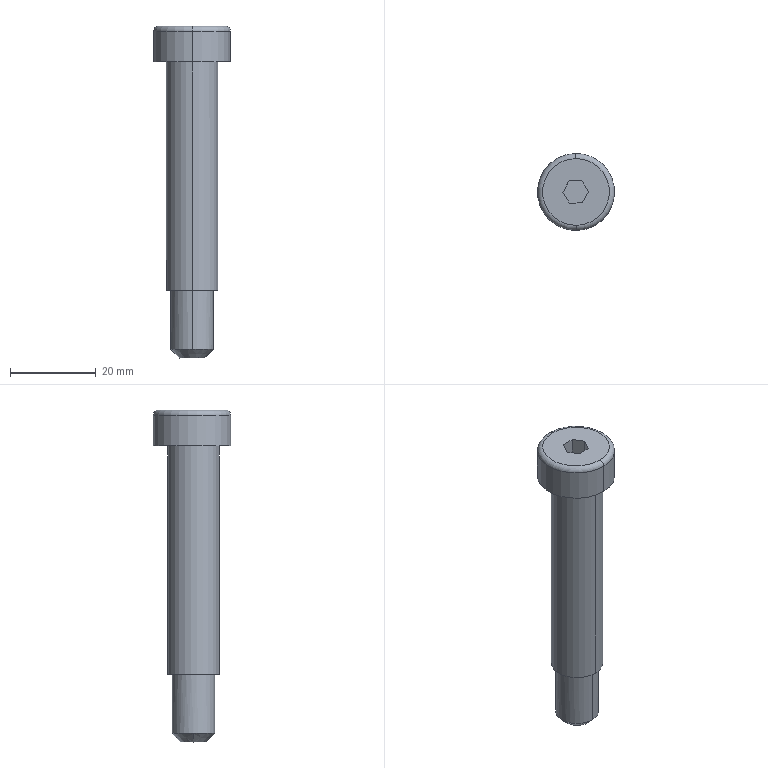Part | SolidWorks | features BaseBody 1 | 1 solid | 21 faces | box 18.001 x 18 x 77.489 mm | volume 9192 mm3 | plane 11 | cylinder 6 | torus 2 | cone 2 | commonest cylinder face diameters 10 x2 12 x2 18 x2
STEP:
#1=CARTESIAN_POINT('',(341.564,206.739,62.122));
#2=VERTEX_POINT('',#1);
#3=CARTESIAN_POINT('',(341.942,188.743,62.122));
#4=VERTEX_POINT('',#3);
#5=CARTESIAN_POINT('',(341.753,197.741,62.122));
#6=DIRECTION('',(-0.0001435,-0.000000521,1.));
#7=DIRECTION('',(0.02104,-0.9998,0.000002497));
#8=AXIS2_PLACEMENT_3D('',#5,#6,#7);
#9=CIRCLE('',#8,9.);
#10=EDGE_CURVE('',#2,#4,#9,.T.);
#11=ORIENTED_EDGE('',*,*,#10,.T.);
#12=CARTESIAN_POINT('',(341.917,189.943,63.322));
#13=VERTEX_POINT('',#12);
#14=CARTESIAN_POINT('',(341.917,189.943,62.122));
#15=DIRECTION('',(-0.9998,-0.02104,-0.0001435));
#16=DIRECTION('',(0.02104,-0.9998,0.));
#17=AXIS2_PLACEMENT_3D('',#14,#15,#16);
#18=CIRCLE('',#17,1.2);
#19=EDGE_CURVE('',#4,#13,#18,.T.);
#20=ORIENTED_EDGE('',*,*,#19,.T.);
#21=CARTESIAN_POINT('',(341.589,205.539,63.322));
#22=VERTEX_POINT('',#21);
#23=CARTESIAN_POINT('',(341.753,197.741,63.322));
#24=DIRECTION('',(-0.0001435,-0.000000521,1.));
#25=DIRECTION('',(0.02104,-0.9998,0.000002497));
#26=AXIS2_PLACEMENT_3D('',#23,#24,#25);
#27=CIRCLE('',#26,7.8);
#28=EDGE_CURVE('',#22,#13,#27,.T.);
#29=ORIENTED_EDGE('',*,*,#28,.F.);
#30=CARTESIAN_POINT('',(341.589,205.539,62.122));
#31=DIRECTION('',(0.9998,0.02104,0.0001435));
#32=DIRECTION('',(-0.02104,0.9998,0.));
#33=AXIS2_PLACEMENT_3D('',#30,#31,#32);
#34=CIRCLE('',#33,1.2);
#35=EDGE_CURVE('',#2,#22,#34,.T.);
#36=ORIENTED_EDGE('',*,*,#35,.F.);
#37=EDGE_LOOP('',(#11,#20,#29,#36));
#38=FACE_OUTER_BOUND('',#37,.T.);
#39=CARTESIAN_POINT('',(341.753,197.741,62.122));
#40=DIRECTION('',(-0.0001435,-0.000000521,1.));
#41=DIRECTION('',(-0.02104,0.9998,-0.000002497));
#42=AXIS2_PLACEMENT_3D('',#39,#40,#41);
#43=TOROIDAL_SURFACE('',#42,7.8,1.2);
#44=ADVANCED_FACE('',(#38),#43,.T.);
#45=CARTESIAN_POINT('',(341.943,188.743,54.922));
#46=VERTEX_POINT('',#45);
#47=CARTESIAN_POINT('',(341.565,206.739,54.922));
#48=VERTEX_POINT('',#47);
#49=CARTESIAN_POINT('',(341.754,197.741,54.922));
#50=DIRECTION('',(0.0001435,0.000000521,-1.));
#51=DIRECTION('',(-0.02104,0.9998,-0.000002497));
#52=AXIS2_PLACEMENT_3D('',#49,#50,#51);
#53=CIRCLE('',#52,9.);
#54=EDGE_CURVE('',#46,#48,#53,.T.);
#55=ORIENTED_EDGE('',*,*,#54,.F.);
#56=CARTESIAN_POINT('',(341.943,188.743,54.922));
#57=DIRECTION('',(-0.0001435,-0.000000521,1.));
#58=VECTOR('',#57,1000.);
#59=LINE('',#56,#58);
#60=EDGE_CURVE('',#46,#4,#59,.T.);
#61=ORIENTED_EDGE('',*,*,#60,.T.);
#62=ORIENTED_EDGE('',*,*,#10,.F.);
#63=CARTESIAN_POINT('',(341.565,206.739,54.922));
#64=DIRECTION('',(-0.0001435,-0.000000521,1.));
#65=VECTOR('',#64,1000.);
#66=LINE('',#63,#65);
#67=EDGE_CURVE('',#48,#2,#66,.T.);
#68=ORIENTED_EDGE('',*,*,#67,.F.);
#69=EDGE_LOOP('',(#55,#61,#62,#68));
#70=FACE_OUTER_BOUND('',#69,.T.);
#71=CARTESIAN_POINT('',(341.754,197.741,54.922));
#72=DIRECTION('',(-0.0001435,-0.000000521,1.));
#73=DIRECTION('',(-0.02104,0.9998,-0.000002497));
#74=AXIS2_PLACEMENT_3D('',#71,#72,#73);
#75=CYLINDRICAL_SURFACE('',#74,9.);
#76=ADVANCED_FACE('',(#70),#75,.T.);
#77=CARTESIAN_POINT('',(341.638,203.402,54.922));
#78=VERTEX_POINT('',#77);
#79=CARTESIAN_POINT('',(341.89,191.405,54.922));
#80=VERTEX_POINT('',#79);
#81=CARTESIAN_POINT('',(341.764,197.404,54.922));
#82=DIRECTION('',(-0.0001435,-0.000000521,1.));
#83=DIRECTION('',(0.02104,-0.9998,0.000002497));
#84=AXIS2_PLACEMENT_3D('',#81,#82,#83);
#85=CIRCLE('',#84,6.);
#86=EDGE_CURVE('',#78,#80,#85,.T.);
#87=ORIENTED_EDGE('',*,*,#86,.F.);
#88=CARTESIAN_POINT('',(341.645,203.402,1.675));
#89=VERTEX_POINT('',#88);
#90=CARTESIAN_POINT('',(341.643,203.402,20.275));
#91=DIRECTION('',(0.0001435,0.000000521,-1.));
#92=VECTOR('',#91,1000.);
#93=LINE('',#90,#92);
#94=EDGE_CURVE('',#78,#89,#93,.T.);
#95=ORIENTED_EDGE('',*,*,#94,.T.);
#96=CARTESIAN_POINT('',(341.898,191.405,1.675));
#97=VERTEX_POINT('',#96);
#98=CARTESIAN_POINT('',(341.771,197.404,1.675));
#99=DIRECTION('',(0.0001435,0.000000521,-1.));
#100=DIRECTION('',(0.02104,-0.9998,0.000002497));
#101=AXIS2_PLACEMENT_3D('',#98,#99,#100);
#102=CIRCLE('',#101,6.);
#103=EDGE_CURVE('',#97,#89,#102,.T.);
#104=ORIENTED_EDGE('',*,*,#103,.F.);
#105=CARTESIAN_POINT('',(341.895,191.405,20.275));
#106=DIRECTION('',(0.0001435,0.000000521,-1.));
#107=VECTOR('',#106,1000.);
#108=LINE('',#105,#107);
#109=EDGE_CURVE('',#80,#97,#108,.T.);
#110=ORIENTED_EDGE('',*,*,#109,.F.);
#111=EDGE_LOOP('',(#87,#95,#104,#110));
#112=FACE_OUTER_BOUND('',#111,.T.);
#113=CARTESIAN_POINT('',(341.769,197.404,20.275));
#114=DIRECTION('',(0.0001435,0.000000521,-1.));
#115=DIRECTION('',(0.02104,-0.9998,0.000002497));
#116=AXIS2_PLACEMENT_3D('',#113,#114,#115);
#117=CYLINDRICAL_SURFACE('',#116,6.);
#118=ADVANCED_FACE('',(#112),#117,.T.);
#119=CARTESIAN_POINT('',(341.666,202.402,1.675));
#120=VERTEX_POINT('',#119);
#121=CARTESIAN_POINT('',(341.877,192.405,1.675));
#122=VERTEX_POINT('',#121);
#123=CARTESIAN_POINT('',(341.771,197.404,1.675));
#124=DIRECTION('',(-0.0001435,-0.000000521,1.));
#125=DIRECTION('',(0.02104,-0.9998,0.000002497));
#126=AXIS2_PLACEMENT_3D('',#123,#124,#125);
#127=CIRCLE('',#126,5.);
#128=EDGE_CURVE('',#120,#122,#127,.T.);
#129=ORIENTED_EDGE('',*,*,#128,.F.);
#130=CARTESIAN_POINT('',(341.668,202.402,-12.165));
#131=VERTEX_POINT('',#130);
#132=CARTESIAN_POINT('',(341.667,202.402,-0.7255));
#133=DIRECTION('',(0.0001435,0.000000521,-1.));
#134=VECTOR('',#133,1000.);
#135=LINE('',#132,#134);
#136=EDGE_CURVE('',#120,#131,#135,.T.);
#137=ORIENTED_EDGE('',*,*,#136,.T.);
#138=CARTESIAN_POINT('',(336.773,197.404,-12.166));
#139=VERTEX_POINT('',#138);
#140=CARTESIAN_POINT('',(341.773,197.404,-12.165));
#141=DIRECTION('',(0.0001435,0.000000521,-1.));
#142=DIRECTION('',(0.02104,-0.9998,0.000002497));
#143=AXIS2_PLACEMENT_3D('',#140,#141,#142);
#144=CIRCLE('',#143,5.);
#145=EDGE_CURVE('',#139,#131,#144,.T.);
#146=ORIENTED_EDGE('',*,*,#145,.F.);
#147=CARTESIAN_POINT('',(341.879,192.405,-12.165));
#148=VERTEX_POINT('',#147);
#149=CARTESIAN_POINT('',(341.773,197.404,-12.165));
#150=DIRECTION('',(0.0001435,0.000000521,-1.));
#151=DIRECTION('',(0.02104,-0.9998,0.000002497));
#152=AXIS2_PLACEMENT_3D('',#149,#150,#151);
#153=CIRCLE('',#152,5.);
#154=EDGE_CURVE('',#148,#139,#153,.T.);
#155=ORIENTED_EDGE('',*,*,#154,.F.);
#156=CARTESIAN_POINT('',(341.877,192.405,-0.7254));
#157=DIRECTION('',(0.0001435,0.000000521,-1.));
#158=VECTOR('',#157,1000.);
#159=LINE('',#156,#158);
#160=EDGE_CURVE('',#122,#148,#159,.T.);
#161=ORIENTED_EDGE('',*,*,#160,.F.);
#162=EDGE_LOOP('',(#129,#137,#146,#155,#161));
#163=FACE_OUTER_BOUND('',#162,.T.);
#164=CARTESIAN_POINT('',(341.772,197.404,-0.7254));
#165=DIRECTION('',(0.0001435,0.000000521,-1.));
#166=DIRECTION('',(0.02104,-0.9998,0.000002497));
#167=AXIS2_PLACEMENT_3D('',#164,#165,#166);
#168=CYLINDRICAL_SURFACE('',#167,5.);
#169=ADVANCED_FACE('',(#163),#168,.T.);
#170=CARTESIAN_POINT('',(338.774,197.404,-14.166));
#171=VERTEX_POINT('',#170);
#172=CARTESIAN_POINT('',(344.774,197.404,-14.165));
#173=VERTEX_POINT('',#172);
#174=CARTESIAN_POINT('',(341.774,197.404,-14.165));
#175=DIRECTION('',(0.0001435,0.000000521,-1.));
#176=DIRECTION('',(-1.,0.,-0.0001435));
#177=AXIS2_PLACEMENT_3D('',#174,#175,#176);
#178=CIRCLE('',#177,3.);
#179=EDGE_CURVE('',#171,#173,#178,.T.);
#180=ORIENTED_EDGE('',*,*,#179,.F.);
#181=CARTESIAN_POINT('',(337.774,197.404,-13.166));
#182=DIRECTION('',(-0.7072,-0.000000369,0.707));
#183=VECTOR('',#182,1000.);
#184=LINE('',#181,#183);
#185=EDGE_CURVE('',#171,#139,#184,.T.);
#186=ORIENTED_EDGE('',*,*,#185,.T.);
#187=ORIENTED_EDGE('',*,*,#145,.T.);
#188=CARTESIAN_POINT('',(346.773,197.404,-12.165));
#189=VERTEX_POINT('',#188);
#190=CARTESIAN_POINT('',(341.773,197.404,-12.165));
#191=DIRECTION('',(0.0001435,0.000000521,-1.));
#192=DIRECTION('',(0.02104,-0.9998,0.000002497));
#193=AXIS2_PLACEMENT_3D('',#190,#191,#192);
#194=CIRCLE('',#193,5.);
#195=EDGE_CURVE('',#131,#189,#194,.T.);
#196=ORIENTED_EDGE('',*,*,#195,.T.);
#197=CARTESIAN_POINT('',(345.774,197.404,-13.165));
#198=DIRECTION('',(0.707,-0.000000369,0.7072));
#199=VECTOR('',#198,1000.);
#200=LINE('',#197,#199);
#201=EDGE_CURVE('',#173,#189,#200,.T.);
#202=ORIENTED_EDGE('',*,*,#201,.F.);
#203=EDGE_LOOP('',(#180,#186,#187,#196,#202));
#204=FACE_OUTER_BOUND('',#203,.T.);
#205=CARTESIAN_POINT('',(341.774,197.404,-13.165));
#206=DIRECTION('',(-0.0001435,-0.000000521,1.));
#207=DIRECTION('',(1.,0.,0.0001435));
#208=AXIS2_PLACEMENT_3D('',#205,#206,#207);
#209=CONICAL_SURFACE('',#208,4.,0.7854);
#210=ADVANCED_FACE('',(#204),#209,.T.);
#211=CARTESIAN_POINT('',(341.774,197.404,-14.165));
#212=DIRECTION('',(0.0001435,0.000000521,-1.));
#213=DIRECTION('',(-1.,0.,-0.0001435));
#214=AXIS2_PLACEMENT_3D('',#211,#212,#213);
#215=CIRCLE('',#214,3.);
#216=EDGE_CURVE('',#173,#171,#215,.T.);
#217=ORIENTED_EDGE('',*,*,#216,.T.);
#218=ORIENTED_EDGE('',*,*,#179,.T.);
#219=EDGE_LOOP('',(#217,#218));
#220=FACE_OUTER_BOUND('',#219,.T.);
#221=CARTESIAN_POINT('',(341.774,197.404,-14.165));
#222=DIRECTION('',(0.0001435,0.000000521,-1.));
#223=DIRECTION('',(0.,-1.,-0.000000521));
#224=AXIS2_PLACEMENT_3D('',#221,#222,#223);
#225=PLANE('',#224);
#226=ADVANCED_FACE('',(#220),#225,.T.);
#227=ORIENTED_EDGE('',*,*,#185,.F.);
#228=ORIENTED_EDGE('',*,*,#216,.F.);
#229=ORIENTED_EDGE('',*,*,#201,.T.);
#230=CARTESIAN_POINT('',(341.773,197.404,-12.165));
#231=DIRECTION('',(0.0001435,0.000000521,-1.));
#232=DIRECTION('',(0.02104,-0.9998,0.000002497));
#233=AXIS2_PLACEMENT_3D('',#230,#231,#232);
#234=CIRCLE('',#233,5.);
#235=EDGE_CURVE('',#189,#148,#234,.T.);
#236=ORIENTED_EDGE('',*,*,#235,.T.);
#237=ORIENTED_EDGE('',*,*,#154,.T.);
#238=EDGE_LOOP('',(#227,#228,#229,#236,#237));
#239=FACE_OUTER_BOUND('',#238,.T.);
#240=CARTESIAN_POINT('',(341.774,197.404,-13.165));
#241=DIRECTION('',(-0.0001435,-0.000000521,1.));
#242=DIRECTION('',(1.,0.,0.0001435));
#243=AXIS2_PLACEMENT_3D('',#240,#241,#242);
#244=CONICAL_SURFACE('',#243,4.,0.7854);
#245=ADVANCED_FACE('',(#239),#244,.T.);
#246=ORIENTED_EDGE('',*,*,#136,.F.);
#247=CARTESIAN_POINT('',(341.771,197.404,1.675));
#248=DIRECTION('',(-0.0001435,-0.000000521,1.));
#249=DIRECTION('',(0.02104,-0.9998,0.000002497));
#250=AXIS2_PLACEMENT_3D('',#247,#248,#249);
#251=CIRCLE('',#250,5.);
#252=EDGE_CURVE('',#122,#120,#251,.T.);
#253=ORIENTED_EDGE('',*,*,#252,.F.);
#254=ORIENTED_EDGE('',*,*,#160,.T.);
#255=ORIENTED_EDGE('',*,*,#235,.F.);
#256=ORIENTED_EDGE('',*,*,#195,.F.);
#257=EDGE_LOOP('',(#246,#253,#254,#255,#256));
#258=FACE_OUTER_BOUND('',#257,.T.);
#259=CARTESIAN_POINT('',(341.772,197.404,-0.7254));
#260=DIRECTION('',(0.0001435,0.000000521,-1.));
#261=DIRECTION('',(0.02104,-0.9998,0.000002497));
#262=AXIS2_PLACEMENT_3D('',#259,#260,#261);
#263=CYLINDRICAL_SURFACE('',#262,5.);
#264=ADVANCED_FACE('',(#258),#263,.T.);
#265=ORIENTED_EDGE('',*,*,#252,.T.);
#266=ORIENTED_EDGE('',*,*,#128,.T.);
#267=EDGE_LOOP('',(#265,#266));
#268=FACE_BOUND('',#267,.T.);
#269=ORIENTED_EDGE('',*,*,#103,.T.);
#270=CARTESIAN_POINT('',(341.771,197.404,1.675));
#271=DIRECTION('',(0.0001435,0.000000521,-1.));
#272=DIRECTION('',(0.02104,-0.9998,0.000002497));
#273=AXIS2_PLACEMENT_3D('',#270,#271,#272);
#274=CIRCLE('',#273,6.);
#275=EDGE_CURVE('',#89,#97,#274,.T.);
#276=ORIENTED_EDGE('',*,*,#275,.T.);
#277=EDGE_LOOP('',(#269,#276));
#278=FACE_OUTER_BOUND('',#277,.T.);
#279=CARTESIAN_POINT('',(341.771,197.404,1.675));
#280=DIRECTION('',(0.0001435,0.000000521,-1.));
#281=DIRECTION('',(0.,-1.,-0.000000521));
#282=AXIS2_PLACEMENT_3D('',#279,#280,#281);
#283=PLANE('',#282);
#284=ADVANCED_FACE('',(#268,#278),#283,.T.);
#285=ORIENTED_EDGE('',*,*,#94,.F.);
#286=CARTESIAN_POINT('',(341.764,197.404,54.922));
#287=DIRECTION('',(-0.0001435,-0.000000521,1.));
#288=DIRECTION('',(0.02104,-0.9998,0.000002497));
#289=AXIS2_PLACEMENT_3D('',#286,#287,#288);
#290=CIRCLE('',#289,6.);
#291=EDGE_CURVE('',#80,#78,#290,.T.);
#292=ORIENTED_EDGE('',*,*,#291,.F.);
#293=ORIENTED_EDGE('',*,*,#109,.T.);
#294=ORIENTED_EDGE('',*,*,#275,.F.);
#295=EDGE_LOOP('',(#285,#292,#293,#294));
#296=FACE_OUTER_BOUND('',#295,.T.);
#297=CARTESIAN_POINT('',(341.769,197.404,20.275));
#298=DIRECTION('',(0.0001435,0.000000521,-1.));
#299=DIRECTION('',(0.02104,-0.9998,0.000002497));
#300=AXIS2_PLACEMENT_3D('',#297,#298,#299);
#301=CYLINDRICAL_SURFACE('',#300,6.);
#302=ADVANCED_FACE('',(#296),#301,.T.);
#303=ORIENTED_EDGE('',*,*,#291,.T.);
#304=ORIENTED_EDGE('',*,*,#86,.T.);
#305=EDGE_LOOP('',(#303,#304));
#306=FACE_BOUND('',#305,.T.);
#307=CARTESIAN_POINT('',(341.754,197.741,54.922));
#308=DIRECTION('',(0.0001435,0.000000521,-1.));
#309=DIRECTION('',(-0.02104,0.9998,-0.000002497));
#310=AXIS2_PLACEMENT_3D('',#307,#308,#309);
#311=CIRCLE('',#310,9.);
#312=EDGE_CURVE('',#48,#46,#311,.T.);
#313=ORIENTED_EDGE('',*,*,#312,.T.);
#314=ORIENTED_EDGE('',*,*,#54,.T.);
#315=EDGE_LOOP('',(#313,#314));
#316=FACE_OUTER_BOUND('',#315,.T.);
#317=CARTESIAN_POINT('',(341.754,197.741,54.922));
#318=DIRECTION('',(0.0001435,0.000000521,-1.));
#319=DIRECTION('',(0.,-1.,-0.000000521));
#320=AXIS2_PLACEMENT_3D('',#317,#318,#319);
#321=PLANE('',#320);
#322=ADVANCED_FACE('',(#306,#316),#321,.T.);
#323=ORIENTED_EDGE('',*,*,#60,.F.);
#324=ORIENTED_EDGE('',*,*,#312,.F.);
#325=ORIENTED_EDGE('',*,*,#67,.T.);
#326=CARTESIAN_POINT('',(341.753,197.741,62.122));
#327=DIRECTION('',(-0.0001435,-0.000000521,1.));
#328=DIRECTION('',(0.02104,-0.9998,0.000002497));
#329=AXIS2_PLACEMENT_3D('',#326,#327,#328);
#330=CIRCLE('',#329,9.);
#331=EDGE_CURVE('',#4,#2,#330,.T.);
#332=ORIENTED_EDGE('',*,*,#331,.F.);
#333=EDGE_LOOP('',(#323,#324,#325,#332));
#334=FACE_OUTER_BOUND('',#333,.T.);
#335=CARTESIAN_POINT('',(341.754,197.741,54.922));
#336=DIRECTION('',(-0.0001435,-0.000000521,1.));
#337=DIRECTION('',(-0.02104,0.9998,-0.000002497));
#338=AXIS2_PLACEMENT_3D('',#335,#336,#337);
#339=CYLINDRICAL_SURFACE('',#338,9.);
#340=ADVANCED_FACE('',(#334),#339,.T.);
#341=ORIENTED_EDGE('',*,*,#19,.F.);
#342=ORIENTED_EDGE('',*,*,#331,.T.);
#343=ORIENTED_EDGE('',*,*,#35,.T.);
#344=CARTESIAN_POINT('',(341.753,197.741,63.322));
#345=DIRECTION('',(-0.0001435,-0.000000521,1.));
#346=DIRECTION('',(0.02104,-0.9998,0.000002497));
#347=AXIS2_PLACEMENT_3D('',#344,#345,#346);
#348=CIRCLE('',#347,7.8);
#349=EDGE_CURVE('',#13,#22,#348,.T.);
#350=ORIENTED_EDGE('',*,*,#349,.F.);
#351=EDGE_LOOP('',(#341,#342,#343,#350));
#352=FACE_OUTER_BOUND('',#351,.T.);
#353=CARTESIAN_POINT('',(341.753,197.741,62.122));
#354=DIRECTION('',(-0.0001435,-0.000000521,1.));
#355=DIRECTION('',(-0.02104,0.9998,-0.000002497));
#356=AXIS2_PLACEMENT_3D('',#353,#354,#355);
#357=TOROIDAL_SURFACE('',#356,7.8,1.2);
#358=ADVANCED_FACE('',(#352),#357,.T.);
#359=CARTESIAN_POINT('',(340.251,195.13,57.322));
#360=VERTEX_POINT('',#359);
#361=CARTESIAN_POINT('',(343.251,195.194,57.322));
#362=VERTEX_POINT('',#361);
#363=CARTESIAN_POINT('',(340.251,195.13,57.322));
#364=DIRECTION('',(0.9998,0.02104,0.0001435));
#365=VECTOR('',#364,1000.);
#366=LINE('',#363,#365);
#367=EDGE_CURVE('',#360,#362,#366,.T.);
#368=ORIENTED_EDGE('',*,*,#367,.T.);
#369=CARTESIAN_POINT('',(344.696,197.823,57.322));
#370=VERTEX_POINT('',#369);
#371=CARTESIAN_POINT('',(343.251,195.194,57.322));
#372=DIRECTION('',(0.4817,0.8764,0.00006956));
#373=VECTOR('',#372,1000.);
#374=LINE('',#371,#373);
#375=EDGE_CURVE('',#362,#370,#374,.T.);
#376=ORIENTED_EDGE('',*,*,#375,.T.);
#377=CARTESIAN_POINT('',(343.142,200.389,57.322));
#378=VERTEX_POINT('',#377);
#379=CARTESIAN_POINT('',(344.696,197.823,57.322));
#380=DIRECTION('',(-0.5181,0.8553,-0.00007389));
#381=VECTOR('',#380,1000.);
#382=LINE('',#379,#381);
#383=EDGE_CURVE('',#370,#378,#382,.T.);
#384=ORIENTED_EDGE('',*,*,#383,.T.);
#385=CARTESIAN_POINT('',(340.142,200.325,57.322));
#386=VERTEX_POINT('',#385);
#387=CARTESIAN_POINT('',(343.142,200.389,57.322));
#388=DIRECTION('',(-0.9998,-0.02104,-0.0001435));
#389=VECTOR('',#388,1000.);
#390=LINE('',#387,#389);
#391=EDGE_CURVE('',#378,#386,#390,.T.);
#392=ORIENTED_EDGE('',*,*,#391,.T.);
#393=CARTESIAN_POINT('',(338.697,197.696,57.322));
#394=VERTEX_POINT('',#393);
#395=CARTESIAN_POINT('',(340.142,200.325,57.322));
#396=DIRECTION('',(-0.4817,-0.8764,-0.00006956));
#397=VECTOR('',#396,1000.);
#398=LINE('',#395,#397);
#399=EDGE_CURVE('',#386,#394,#398,.T.);
#400=ORIENTED_EDGE('',*,*,#399,.T.);
#401=CARTESIAN_POINT('',(338.697,197.696,57.322));
#402=DIRECTION('',(0.5181,-0.8553,0.00007389));
#403=VECTOR('',#402,1000.);
#404=LINE('',#401,#403);
#405=EDGE_CURVE('',#394,#360,#404,.T.);
#406=ORIENTED_EDGE('',*,*,#405,.T.);
#407=EDGE_LOOP('',(#368,#376,#384,#392,#400,#406));
#408=FACE_OUTER_BOUND('',#407,.T.);
#409=CARTESIAN_POINT('',(341.141,226.834,57.322));
#410=DIRECTION('',(-0.0001435,-0.000000521,1.));
#411=DIRECTION('',(-0.003633,1.,0.));
#412=AXIS2_PLACEMENT_3D('',#409,#410,#411);
#413=PLANE('',#412);
#414=ADVANCED_FACE('',(#408),#413,.T.);
#415=CARTESIAN_POINT('',(343.25,195.194,63.322));
#416=VERTEX_POINT('',#415);
#417=CARTESIAN_POINT('',(343.25,195.194,63.322));
#418=DIRECTION('',(0.0001435,0.000000521,-1.));
#419=VECTOR('',#418,1000.);
#420=LINE('',#417,#419);
#421=EDGE_CURVE('',#416,#362,#420,.T.);
#422=ORIENTED_EDGE('',*,*,#421,.T.);
#423=ORIENTED_EDGE('',*,*,#367,.F.);
#424=CARTESIAN_POINT('',(340.251,195.13,63.322));
#425=VERTEX_POINT('',#424);
#426=CARTESIAN_POINT('',(340.251,195.13,63.322));
#427=DIRECTION('',(0.0001435,0.000000521,-1.));
#428=VECTOR('',#427,1000.);
#429=LINE('',#426,#428);
#430=EDGE_CURVE('',#425,#360,#429,.T.);
#431=ORIENTED_EDGE('',*,*,#430,.F.);
#432=CARTESIAN_POINT('',(343.25,195.194,63.322));
#433=DIRECTION('',(-0.9998,-0.02104,-0.0001435));
#434=VECTOR('',#433,1000.);
#435=LINE('',#432,#434);
#436=EDGE_CURVE('',#416,#425,#435,.T.);
#437=ORIENTED_EDGE('',*,*,#436,.F.);
#438=EDGE_LOOP('',(#422,#423,#431,#437));
#439=FACE_OUTER_BOUND('',#438,.T.);
#440=CARTESIAN_POINT('',(343.251,195.194,57.322));
#441=DIRECTION('',(0.02104,-0.9998,0.000002497));
#442=DIRECTION('',(0.,-0.000002498,-1.));
#443=AXIS2_PLACEMENT_3D('',#440,#441,#442);
#444=PLANE('',#443);
#445=ADVANCED_FACE('',(#439),#444,.F.);
#446=CARTESIAN_POINT('',(344.695,197.823,63.322));
#447=VERTEX_POINT('',#446);
#448=CARTESIAN_POINT('',(344.695,197.823,63.322));
#449=DIRECTION('',(0.0001435,0.000000521,-1.));
#450=VECTOR('',#449,1000.);
#451=LINE('',#448,#450);
#452=EDGE_CURVE('',#447,#370,#451,.T.);
#453=ORIENTED_EDGE('',*,*,#452,.T.);
#454=ORIENTED_EDGE('',*,*,#375,.F.);
#455=ORIENTED_EDGE('',*,*,#421,.F.);
#456=CARTESIAN_POINT('',(344.695,197.823,63.322));
#457=DIRECTION('',(-0.4817,-0.8764,-0.00006956));
#458=VECTOR('',#457,1000.);
#459=LINE('',#456,#458);
#460=EDGE_CURVE('',#447,#416,#459,.T.);
#461=ORIENTED_EDGE('',*,*,#460,.F.);
#462=EDGE_LOOP('',(#453,#454,#455,#461));
#463=FACE_OUTER_BOUND('',#462,.T.);
#464=CARTESIAN_POINT('',(344.696,197.823,57.322));
#465=DIRECTION('',(0.8764,-0.4817,0.0001255));
#466=DIRECTION('',(0.,-0.0002605,-1.));
#467=AXIS2_PLACEMENT_3D('',#464,#465,#466);
#468=PLANE('',#467);
#469=ADVANCED_FACE('',(#463),#468,.F.);
#470=CARTESIAN_POINT('',(343.141,200.389,63.322));
#471=VERTEX_POINT('',#470);
#472=CARTESIAN_POINT('',(343.141,200.389,63.322));
#473=DIRECTION('',(0.0001435,0.000000521,-1.));
#474=VECTOR('',#473,1000.);
#475=LINE('',#472,#474);
#476=EDGE_CURVE('',#471,#378,#475,.T.);
#477=ORIENTED_EDGE('',*,*,#476,.T.);
#478=ORIENTED_EDGE('',*,*,#383,.F.);
#479=ORIENTED_EDGE('',*,*,#452,.F.);
#480=CARTESIAN_POINT('',(343.141,200.389,63.322));
#481=DIRECTION('',(0.5181,-0.8553,0.00007389));
#482=VECTOR('',#481,1000.);
#483=LINE('',#480,#482);
#484=EDGE_CURVE('',#471,#447,#483,.T.);
#485=ORIENTED_EDGE('',*,*,#484,.F.);
#486=EDGE_LOOP('',(#477,#478,#479,#485));
#487=FACE_OUTER_BOUND('',#486,.T.);
#488=CARTESIAN_POINT('',(343.142,200.389,57.322));
#489=DIRECTION('',(0.8553,0.5181,0.000123));
#490=DIRECTION('',(0.,0.0002374,-1.));
#491=AXIS2_PLACEMENT_3D('',#488,#489,#490);
#492=PLANE('',#491);
#493=ADVANCED_FACE('',(#487),#492,.F.);
#494=CARTESIAN_POINT('',(340.141,200.325,63.322));
#495=VERTEX_POINT('',#494);
#496=CARTESIAN_POINT('',(340.141,200.325,63.322));
#497=DIRECTION('',(0.0001435,0.000000521,-1.));
#498=VECTOR('',#497,1000.);
#499=LINE('',#496,#498);
#500=EDGE_CURVE('',#495,#386,#499,.T.);
#501=ORIENTED_EDGE('',*,*,#500,.T.);
#502=ORIENTED_EDGE('',*,*,#391,.F.);
#503=ORIENTED_EDGE('',*,*,#476,.F.);
#504=CARTESIAN_POINT('',(340.141,200.325,63.322));
#505=DIRECTION('',(0.9998,0.02104,0.0001435));
#506=VECTOR('',#505,1000.);
#507=LINE('',#504,#506);
#508=EDGE_CURVE('',#495,#471,#507,.T.);
#509=ORIENTED_EDGE('',*,*,#508,.F.);
#510=EDGE_LOOP('',(#501,#502,#503,#509));
#511=FACE_OUTER_BOUND('',#510,.T.);
#512=CARTESIAN_POINT('',(340.142,200.325,57.322));
#513=DIRECTION('',(-0.02104,0.9998,-0.000002497));
#514=DIRECTION('',(-0.0001187,0.,1.));
#515=AXIS2_PLACEMENT_3D('',#512,#513,#514);
#516=PLANE('',#515);
#517=ADVANCED_FACE('',(#511),#516,.F.);
#518=CARTESIAN_POINT('',(338.696,197.696,63.322));
#519=VERTEX_POINT('',#518);
#520=CARTESIAN_POINT('',(338.696,197.696,63.322));
#521=DIRECTION('',(0.0001435,0.000000521,-1.));
#522=VECTOR('',#521,1000.);
#523=LINE('',#520,#522);
#524=EDGE_CURVE('',#519,#394,#523,.T.);
#525=ORIENTED_EDGE('',*,*,#524,.T.);
#526=ORIENTED_EDGE('',*,*,#399,.F.);
#527=ORIENTED_EDGE('',*,*,#500,.F.);
#528=CARTESIAN_POINT('',(338.696,197.696,63.322));
#529=DIRECTION('',(0.4817,0.8764,0.00006956));
#530=VECTOR('',#529,1000.);
#531=LINE('',#528,#530);
#532=EDGE_CURVE('',#519,#495,#531,.T.);
#533=ORIENTED_EDGE('',*,*,#532,.F.);
#534=EDGE_LOOP('',(#525,#526,#527,#533));
#535=FACE_OUTER_BOUND('',#534,.T.);
#536=CARTESIAN_POINT('',(338.697,197.696,57.322));
#537=DIRECTION('',(-0.8764,0.4817,-0.0001255));
#538=DIRECTION('',(-0.0001432,0.,1.));
#539=AXIS2_PLACEMENT_3D('',#536,#537,#538);
#540=PLANE('',#539);
#541=ADVANCED_FACE('',(#535),#540,.F.);
#542=ORIENTED_EDGE('',*,*,#430,.T.);
#543=ORIENTED_EDGE('',*,*,#405,.F.);
#544=ORIENTED_EDGE('',*,*,#524,.F.);
#545=CARTESIAN_POINT('',(340.251,195.13,63.322));
#546=DIRECTION('',(-0.5181,0.8553,-0.00007389));
#547=VECTOR('',#546,1000.);
#548=LINE('',#545,#547);
#549=EDGE_CURVE('',#425,#519,#548,.T.);
#550=ORIENTED_EDGE('',*,*,#549,.F.);
#551=EDGE_LOOP('',(#542,#543,#544,#550));
#552=FACE_OUTER_BOUND('',#551,.T.);
#553=CARTESIAN_POINT('',(340.251,195.13,57.322));
#554=DIRECTION('',(-0.8553,-0.5181,-0.000123));
#555=DIRECTION('',(-0.5181,0.8553,0.));
#556=AXIS2_PLACEMENT_3D('',#553,#554,#555);
#557=PLANE('',#556);
#558=ADVANCED_FACE('',(#552),#557,.F.);
#559=ORIENTED_EDGE('',*,*,#532,.T.);
#560=ORIENTED_EDGE('',*,*,#508,.T.);
#561=ORIENTED_EDGE('',*,*,#484,.T.);
#562=ORIENTED_EDGE('',*,*,#460,.T.);
#563=ORIENTED_EDGE('',*,*,#436,.T.);
#564=ORIENTED_EDGE('',*,*,#549,.T.);
#565=EDGE_LOOP('',(#559,#560,#561,#562,#563,#564));
#566=FACE_BOUND('',#565,.T.);
#567=ORIENTED_EDGE('',*,*,#28,.T.);
#568=ORIENTED_EDGE('',*,*,#349,.T.);
#569=EDGE_LOOP('',(#567,#568));
#570=FACE_OUTER_BOUND('',#569,.T.);
#571=CARTESIAN_POINT('',(341.753,197.741,63.322));
#572=DIRECTION('',(-0.0001435,-0.000000521,1.));
#573=DIRECTION('',(-0.003633,1.,0.));
#574=AXIS2_PLACEMENT_3D('',#571,#572,#573);
#575=PLANE('',#574);
#576=ADVANCED_FACE('',(#566,#570),#575,.T.);
#577=CLOSED_SHELL('',(#44,#76,#118,#169,#210,#226,#245,#264,#284,#302,#322,#340,#358,#414,#445,#469,#493,#517,#541,#558,#576));
#578=MANIFOLD_SOLID_BREP('',#577);
#579=CARTESIAN_POINT('',(0.,0.,0.));
#580=DIRECTION('',(0.,0.,1.));
#581=DIRECTION('',(1.,0.,0.));
#582=AXIS2_PLACEMENT_3D('',#579,#580,#581);
#583=(LENGTH_UNIT()NAMED_UNIT(*)SI_UNIT(.MILLI.,.METRE.));
#584=UNCERTAINTY_MEASURE_WITH_UNIT(LENGTH_MEASURE(0.00001),#583,'','');
#585=(NAMED_UNIT(*)PLANE_ANGLE_UNIT()SI_UNIT($,.RADIAN.));
#586=(NAMED_UNIT(*)SI_UNIT($,.STERADIAN.)SOLID_ANGLE_UNIT());
#587=(GEOMETRIC_REPRESENTATION_CONTEXT(3)GLOBAL_UNCERTAINTY_ASSIGNED_CONTEXT((#584))GLOBAL_UNIT_ASSIGNED_CONTEXT((#583,#585,#586))REPRESENTATION_CONTEXT('',''));
#588=ADVANCED_BREP_SHAPE_REPRESENTATION('',(#578,#582),#587);